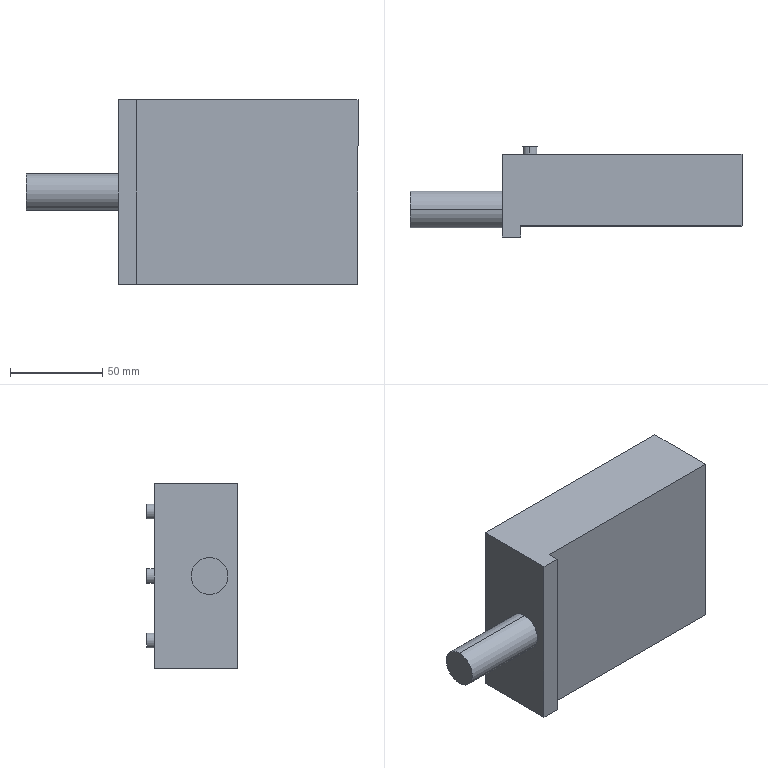Part | SolidWorks | features ICE 6, Extrusion 1, MirrorSolid 1 | 1 solid | 41 faces | box 180 x 49 x 100 mm | volume 529109 mm3 | plane 33 | cylinder 8 | commonest cylinder face diameters 8 x6 20 x2
STEP:
#1=CARTESIAN_POINT('',(-155.,0.,10.));
#2=VERTEX_POINT('',#1);
#3=CARTESIAN_POINT('',(-155.,0.,-10.));
#4=VERTEX_POINT('',#3);
#5=CARTESIAN_POINT('',(-155.,0.,0.));
#6=DIRECTION('',(1.,0.,0.));
#7=DIRECTION('',(0.,0.,-1.));
#8=AXIS2_PLACEMENT_3D('',#5,#6,#7);
#9=CIRCLE('',#8,10.);
#10=EDGE_CURVE('',#2,#4,#9,.T.);
#11=ORIENTED_EDGE('',*,*,#10,.T.);
#12=CARTESIAN_POINT('',(-105.,0.,-10.));
#13=VERTEX_POINT('',#12);
#14=CARTESIAN_POINT('',(-155.,0.,-10.));
#15=DIRECTION('',(1.,0.,0.));
#16=VECTOR('',#15,1000.);
#17=LINE('',#14,#16);
#18=EDGE_CURVE('',#4,#13,#17,.T.);
#19=ORIENTED_EDGE('',*,*,#18,.T.);
#20=CARTESIAN_POINT('',(-105.,0.,10.));
#21=VERTEX_POINT('',#20);
#22=CARTESIAN_POINT('',(-105.,0.,0.));
#23=DIRECTION('',(1.,0.,0.));
#24=DIRECTION('',(0.,0.,-1.));
#25=AXIS2_PLACEMENT_3D('',#22,#23,#24);
#26=CIRCLE('',#25,10.);
#27=EDGE_CURVE('',#21,#13,#26,.T.);
#28=ORIENTED_EDGE('',*,*,#27,.F.);
#29=CARTESIAN_POINT('',(-155.,0.,10.));
#30=DIRECTION('',(1.,0.,0.));
#31=VECTOR('',#30,1000.);
#32=LINE('',#29,#31);
#33=EDGE_CURVE('',#2,#21,#32,.T.);
#34=ORIENTED_EDGE('',*,*,#33,.F.);
#35=EDGE_LOOP('',(#11,#19,#28,#34));
#36=FACE_OUTER_BOUND('',#35,.T.);
#37=CARTESIAN_POINT('',(-155.,0.,0.));
#38=DIRECTION('',(1.,0.,0.));
#39=DIRECTION('',(0.,0.,1.));
#40=AXIS2_PLACEMENT_3D('',#37,#38,#39);
#41=CYLINDRICAL_SURFACE('',#40,10.);
#42=ADVANCED_FACE('',(#36),#41,.T.);
#43=CARTESIAN_POINT('',(-90.,34.,31.));
#44=VERTEX_POINT('',#43);
#45=CARTESIAN_POINT('',(-90.,34.,39.));
#46=VERTEX_POINT('',#45);
#47=CARTESIAN_POINT('',(-90.,34.,35.));
#48=DIRECTION('',(0.,-1.,0.));
#49=DIRECTION('',(0.,0.,1.));
#50=AXIS2_PLACEMENT_3D('',#47,#48,#49);
#51=CIRCLE('',#50,4.);
#52=EDGE_CURVE('',#44,#46,#51,.T.);
#53=ORIENTED_EDGE('',*,*,#52,.T.);
#54=CARTESIAN_POINT('',(-90.,30.,39.));
#55=VERTEX_POINT('',#54);
#56=CARTESIAN_POINT('',(-90.,34.,39.));
#57=DIRECTION('',(0.,-1.,0.));
#58=VECTOR('',#57,1000.);
#59=LINE('',#56,#58);
#60=EDGE_CURVE('',#46,#55,#59,.T.);
#61=ORIENTED_EDGE('',*,*,#60,.T.);
#62=CARTESIAN_POINT('',(-90.,30.,31.));
#63=VERTEX_POINT('',#62);
#64=CARTESIAN_POINT('',(-90.,30.,35.));
#65=DIRECTION('',(0.,-1.,0.));
#66=DIRECTION('',(0.,0.,1.));
#67=AXIS2_PLACEMENT_3D('',#64,#65,#66);
#68=CIRCLE('',#67,4.);
#69=EDGE_CURVE('',#63,#55,#68,.T.);
#70=ORIENTED_EDGE('',*,*,#69,.F.);
#71=CARTESIAN_POINT('',(-90.,34.,31.));
#72=DIRECTION('',(0.,-1.,0.));
#73=VECTOR('',#72,1000.);
#74=LINE('',#71,#73);
#75=EDGE_CURVE('',#44,#63,#74,.T.);
#76=ORIENTED_EDGE('',*,*,#75,.F.);
#77=EDGE_LOOP('',(#53,#61,#70,#76));
#78=FACE_OUTER_BOUND('',#77,.T.);
#79=CARTESIAN_POINT('',(-90.,34.,35.));
#80=DIRECTION('',(0.,-1.,0.));
#81=DIRECTION('',(0.,0.,-1.));
#82=AXIS2_PLACEMENT_3D('',#79,#80,#81);
#83=CYLINDRICAL_SURFACE('',#82,4.);
#84=ADVANCED_FACE('',(#78),#83,.T.);
#85=CARTESIAN_POINT('',(-90.,34.,-4.));
#86=VERTEX_POINT('',#85);
#87=CARTESIAN_POINT('',(-90.,34.,4.));
#88=VERTEX_POINT('',#87);
#89=CARTESIAN_POINT('',(-90.,34.,0.));
#90=DIRECTION('',(0.,-1.,0.));
#91=DIRECTION('',(0.,0.,1.));
#92=AXIS2_PLACEMENT_3D('',#89,#90,#91);
#93=CIRCLE('',#92,4.);
#94=EDGE_CURVE('',#86,#88,#93,.T.);
#95=ORIENTED_EDGE('',*,*,#94,.T.);
#96=CARTESIAN_POINT('',(-90.,30.,4.));
#97=VERTEX_POINT('',#96);
#98=CARTESIAN_POINT('',(-90.,34.,4.));
#99=DIRECTION('',(0.,-1.,0.));
#100=VECTOR('',#99,1000.);
#101=LINE('',#98,#100);
#102=EDGE_CURVE('',#88,#97,#101,.T.);
#103=ORIENTED_EDGE('',*,*,#102,.T.);
#104=CARTESIAN_POINT('',(-90.,30.,-4.));
#105=VERTEX_POINT('',#104);
#106=CARTESIAN_POINT('',(-90.,30.,0.));
#107=DIRECTION('',(0.,-1.,0.));
#108=DIRECTION('',(0.,0.,1.));
#109=AXIS2_PLACEMENT_3D('',#106,#107,#108);
#110=CIRCLE('',#109,4.);
#111=EDGE_CURVE('',#105,#97,#110,.T.);
#112=ORIENTED_EDGE('',*,*,#111,.F.);
#113=CARTESIAN_POINT('',(-90.,34.,-4.));
#114=DIRECTION('',(0.,-1.,0.));
#115=VECTOR('',#114,1000.);
#116=LINE('',#113,#115);
#117=EDGE_CURVE('',#86,#105,#116,.T.);
#118=ORIENTED_EDGE('',*,*,#117,.F.);
#119=EDGE_LOOP('',(#95,#103,#112,#118));
#120=FACE_OUTER_BOUND('',#119,.T.);
#121=CARTESIAN_POINT('',(-90.,34.,0.));
#122=DIRECTION('',(0.,-1.,0.));
#123=DIRECTION('',(0.,0.,-1.));
#124=AXIS2_PLACEMENT_3D('',#121,#122,#123);
#125=CYLINDRICAL_SURFACE('',#124,4.);
#126=ADVANCED_FACE('',(#120),#125,.T.);
#127=CARTESIAN_POINT('',(-90.,34.,-39.));
#128=VERTEX_POINT('',#127);
#129=CARTESIAN_POINT('',(-90.,34.,-31.));
#130=VERTEX_POINT('',#129);
#131=CARTESIAN_POINT('',(-90.,34.,-35.));
#132=DIRECTION('',(0.,-1.,0.));
#133=DIRECTION('',(0.,0.,1.));
#134=AXIS2_PLACEMENT_3D('',#131,#132,#133);
#135=CIRCLE('',#134,4.);
#136=EDGE_CURVE('',#128,#130,#135,.T.);
#137=ORIENTED_EDGE('',*,*,#136,.T.);
#138=CARTESIAN_POINT('',(-90.,30.,-31.));
#139=VERTEX_POINT('',#138);
#140=CARTESIAN_POINT('',(-90.,34.,-31.));
#141=DIRECTION('',(0.,-1.,0.));
#142=VECTOR('',#141,1000.);
#143=LINE('',#140,#142);
#144=EDGE_CURVE('',#130,#139,#143,.T.);
#145=ORIENTED_EDGE('',*,*,#144,.T.);
#146=CARTESIAN_POINT('',(-90.,30.,-39.));
#147=VERTEX_POINT('',#146);
#148=CARTESIAN_POINT('',(-90.,30.,-35.));
#149=DIRECTION('',(0.,-1.,0.));
#150=DIRECTION('',(0.,0.,1.));
#151=AXIS2_PLACEMENT_3D('',#148,#149,#150);
#152=CIRCLE('',#151,4.);
#153=EDGE_CURVE('',#147,#139,#152,.T.);
#154=ORIENTED_EDGE('',*,*,#153,.F.);
#155=CARTESIAN_POINT('',(-90.,34.,-39.));
#156=DIRECTION('',(0.,-1.,0.));
#157=VECTOR('',#156,1000.);
#158=LINE('',#155,#157);
#159=EDGE_CURVE('',#128,#147,#158,.T.);
#160=ORIENTED_EDGE('',*,*,#159,.F.);
#161=EDGE_LOOP('',(#137,#145,#154,#160));
#162=FACE_OUTER_BOUND('',#161,.T.);
#163=CARTESIAN_POINT('',(-90.,34.,-35.));
#164=DIRECTION('',(0.,-1.,0.));
#165=DIRECTION('',(0.,0.,-1.));
#166=AXIS2_PLACEMENT_3D('',#163,#164,#165);
#167=CYLINDRICAL_SURFACE('',#166,4.);
#168=ADVANCED_FACE('',(#162),#167,.T.);
#169=CARTESIAN_POINT('',(-105.,30.,50.));
#170=VERTEX_POINT('',#169);
#171=CARTESIAN_POINT('',(25.,30.,50.));
#172=VERTEX_POINT('',#171);
#173=CARTESIAN_POINT('',(-35.,30.,50.));
#174=DIRECTION('',(1.,0.,0.));
#175=VECTOR('',#174,1000.);
#176=LINE('',#173,#175);
#177=EDGE_CURVE('',#170,#172,#176,.T.);
#178=ORIENTED_EDGE('',*,*,#177,.T.);
#179=CARTESIAN_POINT('',(25.,30.,-50.));
#180=VERTEX_POINT('',#179);
#181=CARTESIAN_POINT('',(25.,30.,50.));
#182=DIRECTION('',(0.,0.,1.));
#183=VECTOR('',#182,1000.);
#184=LINE('',#181,#183);
#185=EDGE_CURVE('',#180,#172,#184,.T.);
#186=ORIENTED_EDGE('',*,*,#185,.F.);
#187=CARTESIAN_POINT('',(-105.,30.,-50.));
#188=VERTEX_POINT('',#187);
#189=CARTESIAN_POINT('',(-35.,30.,-50.));
#190=DIRECTION('',(-1.,0.,0.));
#191=VECTOR('',#190,1000.);
#192=LINE('',#189,#191);
#193=EDGE_CURVE('',#180,#188,#192,.T.);
#194=ORIENTED_EDGE('',*,*,#193,.T.);
#195=CARTESIAN_POINT('',(-105.,30.,-50.));
#196=DIRECTION('',(0.,0.,-1.));
#197=VECTOR('',#196,1000.);
#198=LINE('',#195,#197);
#199=EDGE_CURVE('',#170,#188,#198,.T.);
#200=ORIENTED_EDGE('',*,*,#199,.F.);
#201=EDGE_LOOP('',(#178,#186,#194,#200));
#202=FACE_OUTER_BOUND('',#201,.T.);
#203=ORIENTED_EDGE('',*,*,#111,.T.);
#204=CARTESIAN_POINT('',(-90.,30.,0.));
#205=DIRECTION('',(0.,-1.,0.));
#206=DIRECTION('',(0.,0.,1.));
#207=AXIS2_PLACEMENT_3D('',#204,#205,#206);
#208=CIRCLE('',#207,4.);
#209=EDGE_CURVE('',#97,#105,#208,.T.);
#210=ORIENTED_EDGE('',*,*,#209,.T.);
#211=EDGE_LOOP('',(#203,#210));
#212=FACE_BOUND('',#211,.T.);
#213=ORIENTED_EDGE('',*,*,#153,.T.);
#214=CARTESIAN_POINT('',(-90.,30.,-35.));
#215=DIRECTION('',(0.,-1.,0.));
#216=DIRECTION('',(0.,0.,1.));
#217=AXIS2_PLACEMENT_3D('',#214,#215,#216);
#218=CIRCLE('',#217,4.);
#219=EDGE_CURVE('',#139,#147,#218,.T.);
#220=ORIENTED_EDGE('',*,*,#219,.T.);
#221=EDGE_LOOP('',(#213,#220));
#222=FACE_BOUND('',#221,.T.);
#223=ORIENTED_EDGE('',*,*,#69,.T.);
#224=CARTESIAN_POINT('',(-90.,30.,35.));
#225=DIRECTION('',(0.,-1.,0.));
#226=DIRECTION('',(0.,0.,1.));
#227=AXIS2_PLACEMENT_3D('',#224,#225,#226);
#228=CIRCLE('',#227,4.);
#229=EDGE_CURVE('',#55,#63,#228,.T.);
#230=ORIENTED_EDGE('',*,*,#229,.T.);
#231=EDGE_LOOP('',(#223,#230));
#232=FACE_BOUND('',#231,.T.);
#233=CARTESIAN_POINT('',(0.,30.,0.));
#234=DIRECTION('',(0.,1.,0.));
#235=DIRECTION('',(0.,0.,1.));
#236=AXIS2_PLACEMENT_3D('',#233,#234,#235);
#237=PLANE('',#236);
#238=ADVANCED_FACE('',(#202,#212,#222,#232),#237,.T.);
#239=CARTESIAN_POINT('',(-95.,-9.,-50.));
#240=VERTEX_POINT('',#239);
#241=CARTESIAN_POINT('',(25.,-9.,-50.));
#242=VERTEX_POINT('',#241);
#243=CARTESIAN_POINT('',(-35.,-9.,-50.));
#244=DIRECTION('',(1.,0.,0.));
#245=VECTOR('',#244,1000.);
#246=LINE('',#243,#245);
#247=EDGE_CURVE('',#240,#242,#246,.T.);
#248=ORIENTED_EDGE('',*,*,#247,.F.);
#249=CARTESIAN_POINT('',(-95.,-15.,-50.));
#250=VERTEX_POINT('',#249);
#251=CARTESIAN_POINT('',(-95.,-15.,-50.));
#252=DIRECTION('',(0.,1.,0.));
#253=VECTOR('',#252,1000.);
#254=LINE('',#251,#253);
#255=EDGE_CURVE('',#250,#240,#254,.T.);
#256=ORIENTED_EDGE('',*,*,#255,.F.);
#257=CARTESIAN_POINT('',(-105.,-15.,-50.));
#258=VERTEX_POINT('',#257);
#259=CARTESIAN_POINT('',(-35.,-15.,-50.));
#260=DIRECTION('',(1.,0.,0.));
#261=VECTOR('',#260,1000.);
#262=LINE('',#259,#261);
#263=EDGE_CURVE('',#258,#250,#262,.T.);
#264=ORIENTED_EDGE('',*,*,#263,.F.);
#265=CARTESIAN_POINT('',(-105.,30.,-50.));
#266=DIRECTION('',(0.,-1.,0.));
#267=VECTOR('',#266,1000.);
#268=LINE('',#265,#267);
#269=EDGE_CURVE('',#188,#258,#268,.T.);
#270=ORIENTED_EDGE('',*,*,#269,.F.);
#271=ORIENTED_EDGE('',*,*,#193,.F.);
#272=CARTESIAN_POINT('',(25.,30.,-50.));
#273=DIRECTION('',(0.,1.,0.));
#274=VECTOR('',#273,1000.);
#275=LINE('',#272,#274);
#276=EDGE_CURVE('',#242,#180,#275,.T.);
#277=ORIENTED_EDGE('',*,*,#276,.F.);
#278=EDGE_LOOP('',(#248,#256,#264,#270,#271,#277));
#279=FACE_OUTER_BOUND('',#278,.T.);
#280=CARTESIAN_POINT('',(-35.,30.,-50.));
#281=DIRECTION('',(0.,0.,1.));
#282=DIRECTION('',(1.,0.,0.));
#283=AXIS2_PLACEMENT_3D('',#280,#281,#282);
#284=PLANE('',#283);
#285=ADVANCED_FACE('',(#279),#284,.F.);
#286=CARTESIAN_POINT('',(-95.,-15.,50.));
#287=VERTEX_POINT('',#286);
#288=CARTESIAN_POINT('',(-105.,-15.,50.));
#289=VERTEX_POINT('',#288);
#290=CARTESIAN_POINT('',(-35.,-15.,50.));
#291=DIRECTION('',(-1.,0.,0.));
#292=VECTOR('',#291,1000.);
#293=LINE('',#290,#292);
#294=EDGE_CURVE('',#287,#289,#293,.T.);
#295=ORIENTED_EDGE('',*,*,#294,.F.);
#296=CARTESIAN_POINT('',(-95.,-9.,50.));
#297=VERTEX_POINT('',#296);
#298=CARTESIAN_POINT('',(-95.,-15.,50.));
#299=DIRECTION('',(0.,-1.,0.));
#300=VECTOR('',#299,1000.);
#301=LINE('',#298,#300);
#302=EDGE_CURVE('',#297,#287,#301,.T.);
#303=ORIENTED_EDGE('',*,*,#302,.F.);
#304=CARTESIAN_POINT('',(25.,-9.,50.));
#305=VERTEX_POINT('',#304);
#306=CARTESIAN_POINT('',(-35.,-9.,50.));
#307=DIRECTION('',(-1.,0.,0.));
#308=VECTOR('',#307,1000.);
#309=LINE('',#306,#308);
#310=EDGE_CURVE('',#305,#297,#309,.T.);
#311=ORIENTED_EDGE('',*,*,#310,.F.);
#312=CARTESIAN_POINT('',(25.,30.,50.));
#313=DIRECTION('',(0.,-1.,0.));
#314=VECTOR('',#313,1000.);
#315=LINE('',#312,#314);
#316=EDGE_CURVE('',#172,#305,#315,.T.);
#317=ORIENTED_EDGE('',*,*,#316,.F.);
#318=ORIENTED_EDGE('',*,*,#177,.F.);
#319=CARTESIAN_POINT('',(-105.,30.,50.));
#320=DIRECTION('',(0.,-1.,0.));
#321=VECTOR('',#320,1000.);
#322=LINE('',#319,#321);
#323=EDGE_CURVE('',#170,#289,#322,.T.);
#324=ORIENTED_EDGE('',*,*,#323,.T.);
#325=EDGE_LOOP('',(#295,#303,#311,#317,#318,#324));
#326=FACE_OUTER_BOUND('',#325,.T.);
#327=CARTESIAN_POINT('',(-35.,30.,50.));
#328=DIRECTION('',(0.,0.,-1.));
#329=DIRECTION('',(-1.,0.,0.));
#330=AXIS2_PLACEMENT_3D('',#327,#328,#329);
#331=PLANE('',#330);
#332=ADVANCED_FACE('',(#326),#331,.F.);
#333=CARTESIAN_POINT('',(-95.,-15.,-50.001));
#334=DIRECTION('',(0.,0.,1.));
#335=VECTOR('',#334,1000.);
#336=LINE('',#333,#335);
#337=EDGE_CURVE('',#250,#287,#336,.T.);
#338=ORIENTED_EDGE('',*,*,#337,.T.);
#339=ORIENTED_EDGE('',*,*,#294,.T.);
#340=CARTESIAN_POINT('',(-105.,-15.,50.));
#341=DIRECTION('',(0.,0.,1.));
#342=VECTOR('',#341,1000.);
#343=LINE('',#340,#342);
#344=EDGE_CURVE('',#258,#289,#343,.T.);
#345=ORIENTED_EDGE('',*,*,#344,.F.);
#346=ORIENTED_EDGE('',*,*,#263,.T.);
#347=EDGE_LOOP('',(#338,#339,#345,#346));
#348=FACE_OUTER_BOUND('',#347,.T.);
#349=CARTESIAN_POINT('',(0.,-15.,0.));
#350=DIRECTION('',(0.,-1.,0.));
#351=DIRECTION('',(0.,0.,-1.));
#352=AXIS2_PLACEMENT_3D('',#349,#350,#351);
#353=PLANE('',#352);
#354=ADVANCED_FACE('',(#348),#353,.T.);
#355=ORIENTED_EDGE('',*,*,#344,.T.);
#356=ORIENTED_EDGE('',*,*,#323,.F.);
#357=ORIENTED_EDGE('',*,*,#199,.T.);
#358=ORIENTED_EDGE('',*,*,#269,.T.);
#359=EDGE_LOOP('',(#355,#356,#357,#358));
#360=FACE_OUTER_BOUND('',#359,.T.);
#361=ORIENTED_EDGE('',*,*,#27,.T.);
#362=CARTESIAN_POINT('',(-105.,0.,0.));
#363=DIRECTION('',(1.,0.,0.));
#364=DIRECTION('',(0.,0.,-1.));
#365=AXIS2_PLACEMENT_3D('',#362,#363,#364);
#366=CIRCLE('',#365,10.);
#367=EDGE_CURVE('',#13,#21,#366,.T.);
#368=ORIENTED_EDGE('',*,*,#367,.T.);
#369=EDGE_LOOP('',(#361,#368));
#370=FACE_BOUND('',#369,.T.);
#371=CARTESIAN_POINT('',(-105.,30.,-50.));
#372=DIRECTION('',(1.,0.,0.));
#373=DIRECTION('',(0.,0.,1.));
#374=AXIS2_PLACEMENT_3D('',#371,#372,#373);
#375=PLANE('',#374);
#376=ADVANCED_FACE('',(#360,#370),#375,.F.);
#377=ORIENTED_EDGE('',*,*,#136,.F.);
#378=CARTESIAN_POINT('',(-90.,34.,-35.));
#379=DIRECTION('',(0.,-1.,0.));
#380=DIRECTION('',(0.,0.,1.));
#381=AXIS2_PLACEMENT_3D('',#378,#379,#380);
#382=CIRCLE('',#381,4.);
#383=EDGE_CURVE('',#130,#128,#382,.T.);
#384=ORIENTED_EDGE('',*,*,#383,.F.);
#385=EDGE_LOOP('',(#377,#384));
#386=FACE_OUTER_BOUND('',#385,.T.);
#387=CARTESIAN_POINT('',(-91.913,34.,-33.535));
#388=VERTEX_POINT('',#387);
#389=CARTESIAN_POINT('',(-92.226,34.,-35.924));
#390=VERTEX_POINT('',#389);
#391=CARTESIAN_POINT('',(-91.913,34.,-33.535));
#392=DIRECTION('',(-0.1297,0.,-0.9916));
#393=VECTOR('',#392,1000.);
#394=LINE('',#391,#393);
#395=EDGE_CURVE('',#388,#390,#394,.T.);
#396=ORIENTED_EDGE('',*,*,#395,.T.);
#397=CARTESIAN_POINT('',(-90.312,34.,-37.389));
#398=VERTEX_POINT('',#397);
#399=CARTESIAN_POINT('',(-92.226,34.,-35.924));
#400=DIRECTION('',(0.7939,0.,-0.6081));
#401=VECTOR('',#400,1000.);
#402=LINE('',#399,#401);
#403=EDGE_CURVE('',#390,#398,#402,.T.);
#404=ORIENTED_EDGE('',*,*,#403,.T.);
#405=CARTESIAN_POINT('',(-88.087,34.,-36.465));
#406=VERTEX_POINT('',#405);
#407=CARTESIAN_POINT('',(-90.312,34.,-37.389));
#408=DIRECTION('',(0.9235,0.,0.3835));
#409=VECTOR('',#408,1000.);
#410=LINE('',#407,#409);
#411=EDGE_CURVE('',#398,#406,#410,.T.);
#412=ORIENTED_EDGE('',*,*,#411,.T.);
#413=CARTESIAN_POINT('',(-87.774,34.,-34.076));
#414=VERTEX_POINT('',#413);
#415=CARTESIAN_POINT('',(-88.087,34.,-36.465));
#416=DIRECTION('',(0.1297,0.,0.9916));
#417=VECTOR('',#416,1000.);
#418=LINE('',#415,#417);
#419=EDGE_CURVE('',#406,#414,#418,.T.);
#420=ORIENTED_EDGE('',*,*,#419,.T.);
#421=CARTESIAN_POINT('',(-89.688,34.,-32.611));
#422=VERTEX_POINT('',#421);
#423=CARTESIAN_POINT('',(-87.774,34.,-34.076));
#424=DIRECTION('',(-0.7939,0.,0.6081));
#425=VECTOR('',#424,1000.);
#426=LINE('',#423,#425);
#427=EDGE_CURVE('',#414,#422,#426,.T.);
#428=ORIENTED_EDGE('',*,*,#427,.T.);
#429=CARTESIAN_POINT('',(-89.688,34.,-32.611));
#430=DIRECTION('',(-0.9235,0.,-0.3835));
#431=VECTOR('',#430,1000.);
#432=LINE('',#429,#431);
#433=EDGE_CURVE('',#422,#388,#432,.T.);
#434=ORIENTED_EDGE('',*,*,#433,.T.);
#435=EDGE_LOOP('',(#396,#404,#412,#420,#428,#434));
#436=FACE_BOUND('',#435,.T.);
#437=CARTESIAN_POINT('',(-90.,34.,-35.));
#438=DIRECTION('',(0.,1.,0.));
#439=DIRECTION('',(0.,0.,1.));
#440=AXIS2_PLACEMENT_3D('',#437,#438,#439);
#441=PLANE('',#440);
#442=ADVANCED_FACE('',(#386,#436),#441,.T.);
#443=ORIENTED_EDGE('',*,*,#144,.F.);
#444=ORIENTED_EDGE('',*,*,#383,.T.);
#445=ORIENTED_EDGE('',*,*,#159,.T.);
#446=ORIENTED_EDGE('',*,*,#219,.F.);
#447=EDGE_LOOP('',(#443,#444,#445,#446));
#448=FACE_OUTER_BOUND('',#447,.T.);
#449=CARTESIAN_POINT('',(-90.,34.,-35.));
#450=DIRECTION('',(0.,-1.,0.));
#451=DIRECTION('',(0.,0.,-1.));
#452=AXIS2_PLACEMENT_3D('',#449,#450,#451);
#453=CYLINDRICAL_SURFACE('',#452,4.);
#454=ADVANCED_FACE('',(#448),#453,.T.);
#455=CARTESIAN_POINT('',(-89.688,30.,-32.611));
#456=VERTEX_POINT('',#455);
#457=CARTESIAN_POINT('',(-91.913,30.,-33.535));
#458=VERTEX_POINT('',#457);
#459=CARTESIAN_POINT('',(-89.688,30.,-32.611));
#460=DIRECTION('',(-0.9235,0.,-0.3835));
#461=VECTOR('',#460,1000.);
#462=LINE('',#459,#461);
#463=EDGE_CURVE('',#456,#458,#462,.T.);
#464=ORIENTED_EDGE('',*,*,#463,.T.);
#465=CARTESIAN_POINT('',(-91.913,34.,-33.535));
#466=DIRECTION('',(0.,-1.,0.));
#467=VECTOR('',#466,1000.);
#468=LINE('',#465,#467);
#469=EDGE_CURVE('',#388,#458,#468,.T.);
#470=ORIENTED_EDGE('',*,*,#469,.F.);
#471=ORIENTED_EDGE('',*,*,#433,.F.);
#472=CARTESIAN_POINT('',(-89.688,34.,-32.611));
#473=DIRECTION('',(0.,-1.,0.));
#474=VECTOR('',#473,1000.);
#475=LINE('',#472,#474);
#476=EDGE_CURVE('',#422,#456,#475,.T.);
#477=ORIENTED_EDGE('',*,*,#476,.T.);
#478=EDGE_LOOP('',(#464,#470,#471,#477));
#479=FACE_OUTER_BOUND('',#478,.T.);
#480=CARTESIAN_POINT('',(-89.688,34.,-32.611));
#481=DIRECTION('',(0.3835,0.,-0.9235));
#482=DIRECTION('',(0.9235,0.,0.3835));
#483=AXIS2_PLACEMENT_3D('',#480,#481,#482);
#484=PLANE('',#483);
#485=ADVANCED_FACE('',(#479),#484,.T.);
#486=CARTESIAN_POINT('',(-92.226,30.,-35.924));
#487=VERTEX_POINT('',#486);
#488=CARTESIAN_POINT('',(-91.913,30.,-33.535));
#489=DIRECTION('',(-0.1297,0.,-0.9916));
#490=VECTOR('',#489,1000.);
#491=LINE('',#488,#490);
#492=EDGE_CURVE('',#458,#487,#491,.T.);
#493=ORIENTED_EDGE('',*,*,#492,.T.);
#494=CARTESIAN_POINT('',(-92.226,34.,-35.924));
#495=DIRECTION('',(0.,-1.,0.));
#496=VECTOR('',#495,1000.);
#497=LINE('',#494,#496);
#498=EDGE_CURVE('',#390,#487,#497,.T.);
#499=ORIENTED_EDGE('',*,*,#498,.F.);
#500=ORIENTED_EDGE('',*,*,#395,.F.);
#501=ORIENTED_EDGE('',*,*,#469,.T.);
#502=EDGE_LOOP('',(#493,#499,#500,#501));
#503=FACE_OUTER_BOUND('',#502,.T.);
#504=CARTESIAN_POINT('',(-91.913,34.,-33.535));
#505=DIRECTION('',(0.9916,0.,-0.1297));
#506=DIRECTION('',(0.1297,0.,0.9916));
#507=AXIS2_PLACEMENT_3D('',#504,#505,#506);
#508=PLANE('',#507);
#509=ADVANCED_FACE('',(#503),#508,.T.);
#510=CARTESIAN_POINT('',(-90.312,30.,-37.389));
#511=VERTEX_POINT('',#510);
#512=CARTESIAN_POINT('',(-92.226,30.,-35.924));
#513=DIRECTION('',(0.7939,0.,-0.6081));
#514=VECTOR('',#513,1000.);
#515=LINE('',#512,#514);
#516=EDGE_CURVE('',#487,#511,#515,.T.);
#517=ORIENTED_EDGE('',*,*,#516,.T.);
#518=CARTESIAN_POINT('',(-90.312,34.,-37.389));
#519=DIRECTION('',(0.,-1.,0.));
#520=VECTOR('',#519,1000.);
#521=LINE('',#518,#520);
#522=EDGE_CURVE('',#398,#511,#521,.T.);
#523=ORIENTED_EDGE('',*,*,#522,.F.);
#524=ORIENTED_EDGE('',*,*,#403,.F.);
#525=ORIENTED_EDGE('',*,*,#498,.T.);
#526=EDGE_LOOP('',(#517,#523,#524,#525));
#527=FACE_OUTER_BOUND('',#526,.T.);
#528=CARTESIAN_POINT('',(-92.226,34.,-35.924));
#529=DIRECTION('',(0.6081,0.,0.7939));
#530=DIRECTION('',(-0.7939,0.,0.6081));
#531=AXIS2_PLACEMENT_3D('',#528,#529,#530);
#532=PLANE('',#531);
#533=ADVANCED_FACE('',(#527),#532,.T.);
#534=CARTESIAN_POINT('',(-88.087,30.,-36.465));
#535=VERTEX_POINT('',#534);
#536=CARTESIAN_POINT('',(-90.312,30.,-37.389));
#537=DIRECTION('',(0.9235,0.,0.3835));
#538=VECTOR('',#537,1000.);
#539=LINE('',#536,#538);
#540=EDGE_CURVE('',#511,#535,#539,.T.);
#541=ORIENTED_EDGE('',*,*,#540,.T.);
#542=CARTESIAN_POINT('',(-88.087,34.,-36.465));
#543=DIRECTION('',(0.,-1.,0.));
#544=VECTOR('',#543,1000.);
#545=LINE('',#542,#544);
#546=EDGE_CURVE('',#406,#535,#545,.T.);
#547=ORIENTED_EDGE('',*,*,#546,.F.);
#548=ORIENTED_EDGE('',*,*,#411,.F.);
#549=ORIENTED_EDGE('',*,*,#522,.T.);
#550=EDGE_LOOP('',(#541,#547,#548,#549));
#551=FACE_OUTER_BOUND('',#550,.T.);
#552=CARTESIAN_POINT('',(-90.312,34.,-37.389));
#553=DIRECTION('',(-0.3835,0.,0.9235));
#554=DIRECTION('',(-0.9235,0.,-0.3835));
#555=AXIS2_PLACEMENT_3D('',#552,#553,#554);
#556=PLANE('',#555);
#557=ADVANCED_FACE('',(#551),#556,.T.);
#558=CARTESIAN_POINT('',(-87.774,30.,-34.076));
#559=VERTEX_POINT('',#558);
#560=CARTESIAN_POINT('',(-88.087,30.,-36.465));
#561=DIRECTION('',(0.1297,0.,0.9916));
#562=VECTOR('',#561,1000.);
#563=LINE('',#560,#562);
#564=EDGE_CURVE('',#535,#559,#563,.T.);
#565=ORIENTED_EDGE('',*,*,#564,.T.);
#566=CARTESIAN_POINT('',(-87.774,34.,-34.076));
#567=DIRECTION('',(0.,-1.,0.));
#568=VECTOR('',#567,1000.);
#569=LINE('',#566,#568);
#570=EDGE_CURVE('',#414,#559,#569,.T.);
#571=ORIENTED_EDGE('',*,*,#570,.F.);
#572=ORIENTED_EDGE('',*,*,#419,.F.);
#573=ORIENTED_EDGE('',*,*,#546,.T.);
#574=EDGE_LOOP('',(#565,#571,#572,#573));
#575=FACE_OUTER_BOUND('',#574,.T.);
#576=CARTESIAN_POINT('',(-88.087,34.,-36.465));
#577=DIRECTION('',(-0.9916,0.,0.1297));
#578=DIRECTION('',(-0.1297,0.,-0.9916));
#579=AXIS2_PLACEMENT_3D('',#576,#577,#578);
#580=PLANE('',#579);
#581=ADVANCED_FACE('',(#575),#580,.T.);
#582=CARTESIAN_POINT('',(-87.774,30.,-34.076));
#583=DIRECTION('',(-0.7939,0.,0.6081));
#584=VECTOR('',#583,1000.);
#585=LINE('',#582,#584);
#586=EDGE_CURVE('',#559,#456,#585,.T.);
#587=ORIENTED_EDGE('',*,*,#586,.T.);
#588=ORIENTED_EDGE('',*,*,#476,.F.);
#589=ORIENTED_EDGE('',*,*,#427,.F.);
#590=ORIENTED_EDGE('',*,*,#570,.T.);
#591=EDGE_LOOP('',(#587,#588,#589,#590));
#592=FACE_OUTER_BOUND('',#591,.T.);
#593=CARTESIAN_POINT('',(-87.774,34.,-34.076));
#594=DIRECTION('',(-0.6081,0.,-0.7939));
#595=DIRECTION('',(0.7939,0.,-0.6081));
#596=AXIS2_PLACEMENT_3D('',#593,#594,#595);
#597=PLANE('',#596);
#598=ADVANCED_FACE('',(#592),#597,.T.);
#599=ORIENTED_EDGE('',*,*,#463,.F.);
#600=ORIENTED_EDGE('',*,*,#586,.F.);
#601=ORIENTED_EDGE('',*,*,#564,.F.);
#602=ORIENTED_EDGE('',*,*,#540,.F.);
#603=ORIENTED_EDGE('',*,*,#516,.F.);
#604=ORIENTED_EDGE('',*,*,#492,.F.);
#605=EDGE_LOOP('',(#599,#600,#601,#602,#603,#604));
#606=FACE_OUTER_BOUND('',#605,.T.);
#607=CARTESIAN_POINT('',(-70.,30.,0.));
#608=DIRECTION('',(0.,1.,0.));
#609=DIRECTION('',(0.,0.,1.));
#610=AXIS2_PLACEMENT_3D('',#607,#608,#609);
#611=PLANE('',#610);
#612=ADVANCED_FACE('',(#606),#611,.T.);
#613=ORIENTED_EDGE('',*,*,#94,.F.);
#614=CARTESIAN_POINT('',(-90.,34.,0.));
#615=DIRECTION('',(0.,-1.,0.));
#616=DIRECTION('',(0.,0.,1.));
#617=AXIS2_PLACEMENT_3D('',#614,#615,#616);
#618=CIRCLE('',#617,4.);
#619=EDGE_CURVE('',#88,#86,#618,.T.);
#620=ORIENTED_EDGE('',*,*,#619,.F.);
#621=EDGE_LOOP('',(#613,#620));
#622=FACE_OUTER_BOUND('',#621,.T.);
#623=CARTESIAN_POINT('',(-91.913,34.,1.47));
#624=VERTEX_POINT('',#623);
#625=CARTESIAN_POINT('',(-92.23,34.,-0.9217));
#626=VERTEX_POINT('',#625);
#627=CARTESIAN_POINT('',(-91.913,34.,1.47));
#628=DIRECTION('',(-0.1313,0.,-0.9913));
#629=VECTOR('',#628,1000.);
#630=LINE('',#627,#629);
#631=EDGE_CURVE('',#624,#626,#630,.T.);
#632=ORIENTED_EDGE('',*,*,#631,.T.);
#633=CARTESIAN_POINT('',(-90.317,34.,-2.392));
#634=VERTEX_POINT('',#633);
#635=CARTESIAN_POINT('',(-92.23,34.,-0.9217));
#636=DIRECTION('',(0.7929,0.,-0.6094));
#637=VECTOR('',#636,1000.);
#638=LINE('',#635,#637);
#639=EDGE_CURVE('',#626,#634,#638,.T.);
#640=ORIENTED_EDGE('',*,*,#639,.T.);
#641=CARTESIAN_POINT('',(-88.087,34.,-1.47));
#642=VERTEX_POINT('',#641);
#643=CARTESIAN_POINT('',(-90.317,34.,-2.392));
#644=DIRECTION('',(0.9242,0.,0.382));
#645=VECTOR('',#644,1000.);
#646=LINE('',#643,#645);
#647=EDGE_CURVE('',#634,#642,#646,.T.);
#648=ORIENTED_EDGE('',*,*,#647,.T.);
#649=CARTESIAN_POINT('',(-87.77,34.,0.9217));
#650=VERTEX_POINT('',#649);
#651=CARTESIAN_POINT('',(-88.087,34.,-1.47));
#652=DIRECTION('',(0.1313,0.,0.9913));
#653=VECTOR('',#652,1000.);
#654=LINE('',#651,#653);
#655=EDGE_CURVE('',#642,#650,#654,.T.);
#656=ORIENTED_EDGE('',*,*,#655,.T.);
#657=CARTESIAN_POINT('',(-89.683,34.,2.392));
#658=VERTEX_POINT('',#657);
#659=CARTESIAN_POINT('',(-87.77,34.,0.9217));
#660=DIRECTION('',(-0.7929,0.,0.6094));
#661=VECTOR('',#660,1000.);
#662=LINE('',#659,#661);
#663=EDGE_CURVE('',#650,#658,#662,.T.);
#664=ORIENTED_EDGE('',*,*,#663,.T.);
#665=CARTESIAN_POINT('',(-89.683,34.,2.392));
#666=DIRECTION('',(-0.9242,0.,-0.382));
#667=VECTOR('',#666,1000.);
#668=LINE('',#665,#667);
#669=EDGE_CURVE('',#658,#624,#668,.T.);
#670=ORIENTED_EDGE('',*,*,#669,.T.);
#671=EDGE_LOOP('',(#632,#640,#648,#656,#664,#670));
#672=FACE_BOUND('',#671,.T.);
#673=CARTESIAN_POINT('',(-90.,34.,0.));
#674=DIRECTION('',(0.,1.,0.));
#675=DIRECTION('',(0.,0.,1.));
#676=AXIS2_PLACEMENT_3D('',#673,#674,#675);
#677=PLANE('',#676);
#678=ADVANCED_FACE('',(#622,#672),#677,.T.);
#679=ORIENTED_EDGE('',*,*,#102,.F.);
#680=ORIENTED_EDGE('',*,*,#619,.T.);
#681=ORIENTED_EDGE('',*,*,#117,.T.);
#682=ORIENTED_EDGE('',*,*,#209,.F.);
#683=EDGE_LOOP('',(#679,#680,#681,#682));
#684=FACE_OUTER_BOUND('',#683,.T.);
#685=CARTESIAN_POINT('',(-90.,34.,0.));
#686=DIRECTION('',(0.,-1.,0.));
#687=DIRECTION('',(0.,0.,-1.));
#688=AXIS2_PLACEMENT_3D('',#685,#686,#687);
#689=CYLINDRICAL_SURFACE('',#688,4.);
#690=ADVANCED_FACE('',(#684),#689,.T.);
#691=CARTESIAN_POINT('',(-89.683,30.,2.392));
#692=VERTEX_POINT('',#691);
#693=CARTESIAN_POINT('',(-91.913,30.,1.47));
#694=VERTEX_POINT('',#693);
#695=CARTESIAN_POINT('',(-89.683,30.,2.392));
#696=DIRECTION('',(-0.9242,0.,-0.382));
#697=VECTOR('',#696,1000.);
#698=LINE('',#695,#697);
#699=EDGE_CURVE('',#692,#694,#698,.T.);
#700=ORIENTED_EDGE('',*,*,#699,.T.);
#701=CARTESIAN_POINT('',(-91.913,34.,1.47));
#702=DIRECTION('',(0.,-1.,0.));
#703=VECTOR('',#702,1000.);
#704=LINE('',#701,#703);
#705=EDGE_CURVE('',#624,#694,#704,.T.);
#706=ORIENTED_EDGE('',*,*,#705,.F.);
#707=ORIENTED_EDGE('',*,*,#669,.F.);
#708=CARTESIAN_POINT('',(-89.683,34.,2.392));
#709=DIRECTION('',(0.,-1.,0.));
#710=VECTOR('',#709,1000.);
#711=LINE('',#708,#710);
#712=EDGE_CURVE('',#658,#692,#711,.T.);
#713=ORIENTED_EDGE('',*,*,#712,.T.);
#714=EDGE_LOOP('',(#700,#706,#707,#713));
#715=FACE_OUTER_BOUND('',#714,.T.);
#716=CARTESIAN_POINT('',(-89.683,34.,2.392));
#717=DIRECTION('',(0.382,0.,-0.9242));
#718=DIRECTION('',(0.9242,0.,0.382));
#719=AXIS2_PLACEMENT_3D('',#716,#717,#718);
#720=PLANE('',#719);
#721=ADVANCED_FACE('',(#715),#720,.T.);
#722=CARTESIAN_POINT('',(-92.23,30.,-0.9217));
#723=VERTEX_POINT('',#722);
#724=CARTESIAN_POINT('',(-91.913,30.,1.47));
#725=DIRECTION('',(-0.1313,0.,-0.9913));
#726=VECTOR('',#725,1000.);
#727=LINE('',#724,#726);
#728=EDGE_CURVE('',#694,#723,#727,.T.);
#729=ORIENTED_EDGE('',*,*,#728,.T.);
#730=CARTESIAN_POINT('',(-92.23,34.,-0.9217));
#731=DIRECTION('',(0.,-1.,0.));
#732=VECTOR('',#731,1000.);
#733=LINE('',#730,#732);
#734=EDGE_CURVE('',#626,#723,#733,.T.);
#735=ORIENTED_EDGE('',*,*,#734,.F.);
#736=ORIENTED_EDGE('',*,*,#631,.F.);
#737=ORIENTED_EDGE('',*,*,#705,.T.);
#738=EDGE_LOOP('',(#729,#735,#736,#737));
#739=FACE_OUTER_BOUND('',#738,.T.);
#740=CARTESIAN_POINT('',(-91.913,34.,1.47));
#741=DIRECTION('',(0.9913,0.,-0.1313));
#742=DIRECTION('',(0.1313,0.,0.9913));
#743=AXIS2_PLACEMENT_3D('',#740,#741,#742);
#744=PLANE('',#743);
#745=ADVANCED_FACE('',(#739),#744,.T.);
#746=CARTESIAN_POINT('',(-90.317,30.,-2.392));
#747=VERTEX_POINT('',#746);
#748=CARTESIAN_POINT('',(-92.23,30.,-0.9217));
#749=DIRECTION('',(0.7929,0.,-0.6094));
#750=VECTOR('',#749,1000.);
#751=LINE('',#748,#750);
#752=EDGE_CURVE('',#723,#747,#751,.T.);
#753=ORIENTED_EDGE('',*,*,#752,.T.);
#754=CARTESIAN_POINT('',(-90.317,34.,-2.392));
#755=DIRECTION('',(0.,-1.,0.));
#756=VECTOR('',#755,1000.);
#757=LINE('',#754,#756);
#758=EDGE_CURVE('',#634,#747,#757,.T.);
#759=ORIENTED_EDGE('',*,*,#758,.F.);
#760=ORIENTED_EDGE('',*,*,#639,.F.);
#761=ORIENTED_EDGE('',*,*,#734,.T.);
#762=EDGE_LOOP('',(#753,#759,#760,#761));
#763=FACE_OUTER_BOUND('',#762,.T.);
#764=CARTESIAN_POINT('',(-92.23,34.,-0.9217));
#765=DIRECTION('',(0.6094,0.,0.7929));
#766=DIRECTION('',(-0.7929,0.,0.6094));
#767=AXIS2_PLACEMENT_3D('',#764,#765,#766);
#768=PLANE('',#767);
#769=ADVANCED_FACE('',(#763),#768,.T.);
#770=CARTESIAN_POINT('',(-88.087,30.,-1.47));
#771=VERTEX_POINT('',#770);
#772=CARTESIAN_POINT('',(-90.317,30.,-2.392));
#773=DIRECTION('',(0.9242,0.,0.382));
#774=VECTOR('',#773,1000.);
#775=LINE('',#772,#774);
#776=EDGE_CURVE('',#747,#771,#775,.T.);
#777=ORIENTED_EDGE('',*,*,#776,.T.);
#778=CARTESIAN_POINT('',(-88.087,34.,-1.47));
#779=DIRECTION('',(0.,-1.,0.));
#780=VECTOR('',#779,1000.);
#781=LINE('',#778,#780);
#782=EDGE_CURVE('',#642,#771,#781,.T.);
#783=ORIENTED_EDGE('',*,*,#782,.F.);
#784=ORIENTED_EDGE('',*,*,#647,.F.);
#785=ORIENTED_EDGE('',*,*,#758,.T.);
#786=EDGE_LOOP('',(#777,#783,#784,#785));
#787=FACE_OUTER_BOUND('',#786,.T.);
#788=CARTESIAN_POINT('',(-90.317,34.,-2.392));
#789=DIRECTION('',(-0.382,0.,0.9242));
#790=DIRECTION('',(-0.9242,0.,-0.382));
#791=AXIS2_PLACEMENT_3D('',#788,#789,#790);
#792=PLANE('',#791);
#793=ADVANCED_FACE('',(#787),#792,.T.);
#794=CARTESIAN_POINT('',(-87.77,30.,0.9217));
#795=VERTEX_POINT('',#794);
#796=CARTESIAN_POINT('',(-88.087,30.,-1.47));
#797=DIRECTION('',(0.1313,0.,0.9913));
#798=VECTOR('',#797,1000.);
#799=LINE('',#796,#798);
#800=EDGE_CURVE('',#771,#795,#799,.T.);
#801=ORIENTED_EDGE('',*,*,#800,.T.);
#802=CARTESIAN_POINT('',(-87.77,34.,0.9217));
#803=DIRECTION('',(0.,-1.,0.));
#804=VECTOR('',#803,1000.);
#805=LINE('',#802,#804);
#806=EDGE_CURVE('',#650,#795,#805,.T.);
#807=ORIENTED_EDGE('',*,*,#806,.F.);
#808=ORIENTED_EDGE('',*,*,#655,.F.);
#809=ORIENTED_EDGE('',*,*,#782,.T.);
#810=EDGE_LOOP('',(#801,#807,#808,#809));
#811=FACE_OUTER_BOUND('',#810,.T.);
#812=CARTESIAN_POINT('',(-88.087,34.,-1.47));
#813=DIRECTION('',(-0.9913,0.,0.1313));
#814=DIRECTION('',(-0.1313,0.,-0.9913));
#815=AXIS2_PLACEMENT_3D('',#812,#813,#814);
#816=PLANE('',#815);
#817=ADVANCED_FACE('',(#811),#816,.T.);
#818=CARTESIAN_POINT('',(-87.77,30.,0.9217));
#819=DIRECTION('',(-0.7929,0.,0.6094));
#820=VECTOR('',#819,1000.);
#821=LINE('',#818,#820);
#822=EDGE_CURVE('',#795,#692,#821,.T.);
#823=ORIENTED_EDGE('',*,*,#822,.T.);
#824=ORIENTED_EDGE('',*,*,#712,.F.);
#825=ORIENTED_EDGE('',*,*,#663,.F.);
#826=ORIENTED_EDGE('',*,*,#806,.T.);
#827=EDGE_LOOP('',(#823,#824,#825,#826));
#828=FACE_OUTER_BOUND('',#827,.T.);
#829=CARTESIAN_POINT('',(-87.77,34.,0.9217));
#830=DIRECTION('',(-0.6094,0.,-0.7929));
#831=DIRECTION('',(0.7929,0.,-0.6094));
#832=AXIS2_PLACEMENT_3D('',#829,#830,#831);
#833=PLANE('',#832);
#834=ADVANCED_FACE('',(#828),#833,.T.);
#835=ORIENTED_EDGE('',*,*,#699,.F.);
#836=ORIENTED_EDGE('',*,*,#822,.F.);
#837=ORIENTED_EDGE('',*,*,#800,.F.);
#838=ORIENTED_EDGE('',*,*,#776,.F.);
#839=ORIENTED_EDGE('',*,*,#752,.F.);
#840=ORIENTED_EDGE('',*,*,#728,.F.);
#841=EDGE_LOOP('',(#835,#836,#837,#838,#839,#840));
#842=FACE_OUTER_BOUND('',#841,.T.);
#843=CARTESIAN_POINT('',(-70.,30.,0.));
#844=DIRECTION('',(0.,1.,0.));
#845=DIRECTION('',(0.,0.,1.));
#846=AXIS2_PLACEMENT_3D('',#843,#844,#845);
#847=PLANE('',#846);
#848=ADVANCED_FACE('',(#842),#847,.T.);
#849=ORIENTED_EDGE('',*,*,#52,.F.);
#850=CARTESIAN_POINT('',(-90.,34.,35.));
#851=DIRECTION('',(0.,-1.,0.));
#852=DIRECTION('',(0.,0.,1.));
#853=AXIS2_PLACEMENT_3D('',#850,#851,#852);
#854=CIRCLE('',#853,4.);
#855=EDGE_CURVE('',#46,#44,#854,.T.);
#856=ORIENTED_EDGE('',*,*,#855,.F.);
#857=EDGE_LOOP('',(#849,#856));
#858=FACE_OUTER_BOUND('',#857,.T.);
#859=CARTESIAN_POINT('',(-91.913,34.,37.035));
#860=VERTEX_POINT('',#859);
#861=CARTESIAN_POINT('',(-92.719,34.,34.361));
#862=VERTEX_POINT('',#861);
#863=CARTESIAN_POINT('',(-91.913,34.,37.035));
#864=DIRECTION('',(-0.2886,0.,-0.9575));
#865=VECTOR('',#864,1000.);
#866=LINE('',#863,#865);
#867=EDGE_CURVE('',#860,#862,#866,.T.);
#868=ORIENTED_EDGE('',*,*,#867,.T.);
#869=CARTESIAN_POINT('',(-90.806,34.,32.326));
#870=VERTEX_POINT('',#869);
#871=CARTESIAN_POINT('',(-92.719,34.,34.361));
#872=DIRECTION('',(0.6849,0.,-0.7286));
#873=VECTOR('',#872,1000.);
#874=LINE('',#871,#873);
#875=EDGE_CURVE('',#862,#870,#874,.T.);
#876=ORIENTED_EDGE('',*,*,#875,.T.);
#877=CARTESIAN_POINT('',(-88.087,34.,32.965));
#878=VERTEX_POINT('',#877);
#879=CARTESIAN_POINT('',(-90.806,34.,32.326));
#880=DIRECTION('',(0.9735,0.,0.2288));
#881=VECTOR('',#880,1000.);
#882=LINE('',#879,#881);
#883=EDGE_CURVE('',#870,#878,#882,.T.);
#884=ORIENTED_EDGE('',*,*,#883,.T.);
#885=CARTESIAN_POINT('',(-87.281,34.,35.639));
#886=VERTEX_POINT('',#885);
#887=CARTESIAN_POINT('',(-88.087,34.,32.965));
#888=DIRECTION('',(0.2886,0.,0.9575));
#889=VECTOR('',#888,1000.);
#890=LINE('',#887,#889);
#891=EDGE_CURVE('',#878,#886,#890,.T.);
#892=ORIENTED_EDGE('',*,*,#891,.T.);
#893=CARTESIAN_POINT('',(-89.194,34.,37.674));
#894=VERTEX_POINT('',#893);
#895=CARTESIAN_POINT('',(-87.281,34.,35.639));
#896=DIRECTION('',(-0.6849,0.,0.7286));
#897=VECTOR('',#896,1000.);
#898=LINE('',#895,#897);
#899=EDGE_CURVE('',#886,#894,#898,.T.);
#900=ORIENTED_EDGE('',*,*,#899,.T.);
#901=CARTESIAN_POINT('',(-89.194,34.,37.674));
#902=DIRECTION('',(-0.9735,0.,-0.2288));
#903=VECTOR('',#902,1000.);
#904=LINE('',#901,#903);
#905=EDGE_CURVE('',#894,#860,#904,.T.);
#906=ORIENTED_EDGE('',*,*,#905,.T.);
#907=EDGE_LOOP('',(#868,#876,#884,#892,#900,#906));
#908=FACE_BOUND('',#907,.T.);
#909=CARTESIAN_POINT('',(-90.,34.,35.));
#910=DIRECTION('',(0.,1.,0.));
#911=DIRECTION('',(0.,0.,1.));
#912=AXIS2_PLACEMENT_3D('',#909,#910,#911);
#913=PLANE('',#912);
#914=ADVANCED_FACE('',(#858,#908),#913,.T.);
#915=ORIENTED_EDGE('',*,*,#60,.F.);
#916=ORIENTED_EDGE('',*,*,#855,.T.);
#917=ORIENTED_EDGE('',*,*,#75,.T.);
#918=ORIENTED_EDGE('',*,*,#229,.F.);
#919=EDGE_LOOP('',(#915,#916,#917,#918));
#920=FACE_OUTER_BOUND('',#919,.T.);
#921=CARTESIAN_POINT('',(-90.,34.,35.));
#922=DIRECTION('',(0.,-1.,0.));
#923=DIRECTION('',(0.,0.,-1.));
#924=AXIS2_PLACEMENT_3D('',#921,#922,#923);
#925=CYLINDRICAL_SURFACE('',#924,4.);
#926=ADVANCED_FACE('',(#920),#925,.T.);
#927=CARTESIAN_POINT('',(-89.194,30.,37.674));
#928=VERTEX_POINT('',#927);
#929=CARTESIAN_POINT('',(-91.913,30.,37.035));
#930=VERTEX_POINT('',#929);
#931=CARTESIAN_POINT('',(-89.194,30.,37.674));
#932=DIRECTION('',(-0.9735,0.,-0.2288));
#933=VECTOR('',#932,1000.);
#934=LINE('',#931,#933);
#935=EDGE_CURVE('',#928,#930,#934,.T.);
#936=ORIENTED_EDGE('',*,*,#935,.T.);
#937=CARTESIAN_POINT('',(-91.913,34.,37.035));
#938=DIRECTION('',(0.,-1.,0.));
#939=VECTOR('',#938,1000.);
#940=LINE('',#937,#939);
#941=EDGE_CURVE('',#860,#930,#940,.T.);
#942=ORIENTED_EDGE('',*,*,#941,.F.);
#943=ORIENTED_EDGE('',*,*,#905,.F.);
#944=CARTESIAN_POINT('',(-89.194,34.,37.674));
#945=DIRECTION('',(0.,-1.,0.));
#946=VECTOR('',#945,1000.);
#947=LINE('',#944,#946);
#948=EDGE_CURVE('',#894,#928,#947,.T.);
#949=ORIENTED_EDGE('',*,*,#948,.T.);
#950=EDGE_LOOP('',(#936,#942,#943,#949));
#951=FACE_OUTER_BOUND('',#950,.T.);
#952=CARTESIAN_POINT('',(-89.194,34.,37.674));
#953=DIRECTION('',(0.2288,0.,-0.9735));
#954=DIRECTION('',(0.9735,0.,0.2288));
#955=AXIS2_PLACEMENT_3D('',#952,#953,#954);
#956=PLANE('',#955);
#957=ADVANCED_FACE('',(#951),#956,.T.);
#958=CARTESIAN_POINT('',(-92.719,30.,34.361));
#959=VERTEX_POINT('',#958);
#960=CARTESIAN_POINT('',(-91.913,30.,37.035));
#961=DIRECTION('',(-0.2886,0.,-0.9575));
#962=VECTOR('',#961,1000.);
#963=LINE('',#960,#962);
#964=EDGE_CURVE('',#930,#959,#963,.T.);
#965=ORIENTED_EDGE('',*,*,#964,.T.);
#966=CARTESIAN_POINT('',(-92.719,34.,34.361));
#967=DIRECTION('',(0.,-1.,0.));
#968=VECTOR('',#967,1000.);
#969=LINE('',#966,#968);
#970=EDGE_CURVE('',#862,#959,#969,.T.);
#971=ORIENTED_EDGE('',*,*,#970,.F.);
#972=ORIENTED_EDGE('',*,*,#867,.F.);
#973=ORIENTED_EDGE('',*,*,#941,.T.);
#974=EDGE_LOOP('',(#965,#971,#972,#973));
#975=FACE_OUTER_BOUND('',#974,.T.);
#976=CARTESIAN_POINT('',(-91.913,34.,37.035));
#977=DIRECTION('',(0.9575,0.,-0.2886));
#978=DIRECTION('',(0.2886,0.,0.9575));
#979=AXIS2_PLACEMENT_3D('',#976,#977,#978);
#980=PLANE('',#979);
#981=ADVANCED_FACE('',(#975),#980,.T.);
#982=CARTESIAN_POINT('',(-90.806,30.,32.326));
#983=VERTEX_POINT('',#982);
#984=CARTESIAN_POINT('',(-92.719,30.,34.361));
#985=DIRECTION('',(0.6849,0.,-0.7286));
#986=VECTOR('',#985,1000.);
#987=LINE('',#984,#986);
#988=EDGE_CURVE('',#959,#983,#987,.T.);
#989=ORIENTED_EDGE('',*,*,#988,.T.);
#990=CARTESIAN_POINT('',(-90.806,34.,32.326));
#991=DIRECTION('',(0.,-1.,0.));
#992=VECTOR('',#991,1000.);
#993=LINE('',#990,#992);
#994=EDGE_CURVE('',#870,#983,#993,.T.);
#995=ORIENTED_EDGE('',*,*,#994,.F.);
#996=ORIENTED_EDGE('',*,*,#875,.F.);
#997=ORIENTED_EDGE('',*,*,#970,.T.);
#998=EDGE_LOOP('',(#989,#995,#996,#997));
#999=FACE_OUTER_BOUND('',#998,.T.);
#1000=CARTESIAN_POINT('',(-92.719,34.,34.361));
#1001=DIRECTION('',(0.7286,0.,0.6849));
#1002=DIRECTION('',(-0.6849,0.,0.7286));
#1003=AXIS2_PLACEMENT_3D('',#1000,#1001,#1002);
#1004=PLANE('',#1003);
#1005=ADVANCED_FACE('',(#999),#1004,.T.);
#1006=CARTESIAN_POINT('',(-88.087,30.,32.965));
#1007=VERTEX_POINT('',#1006);
#1008=CARTESIAN_POINT('',(-90.806,30.,32.326));
#1009=DIRECTION('',(0.9735,0.,0.2288));
#1010=VECTOR('',#1009,1000.);
#1011=LINE('',#1008,#1010);
#1012=EDGE_CURVE('',#983,#1007,#1011,.T.);
#1013=ORIENTED_EDGE('',*,*,#1012,.T.);
#1014=CARTESIAN_POINT('',(-88.087,34.,32.965));
#1015=DIRECTION('',(0.,-1.,0.));
#1016=VECTOR('',#1015,1000.);
#1017=LINE('',#1014,#1016);
#1018=EDGE_CURVE('',#878,#1007,#1017,.T.);
#1019=ORIENTED_EDGE('',*,*,#1018,.F.);
#1020=ORIENTED_EDGE('',*,*,#883,.F.);
#1021=ORIENTED_EDGE('',*,*,#994,.T.);
#1022=EDGE_LOOP('',(#1013,#1019,#1020,#1021));
#1023=FACE_OUTER_BOUND('',#1022,.T.);
#1024=CARTESIAN_POINT('',(-90.806,34.,32.326));
#1025=DIRECTION('',(-0.2288,0.,0.9735));
#1026=DIRECTION('',(-0.9735,0.,-0.2288));
#1027=AXIS2_PLACEMENT_3D('',#1024,#1025,#1026);
#1028=PLANE('',#1027);
#1029=ADVANCED_FACE('',(#1023),#1028,.T.);
#1030=CARTESIAN_POINT('',(-87.281,30.,35.639));
#1031=VERTEX_POINT('',#1030);
#1032=CARTESIAN_POINT('',(-88.087,30.,32.965));
#1033=DIRECTION('',(0.2886,0.,0.9575));
#1034=VECTOR('',#1033,1000.);
#1035=LINE('',#1032,#1034);
#1036=EDGE_CURVE('',#1007,#1031,#1035,.T.);
#1037=ORIENTED_EDGE('',*,*,#1036,.T.);
#1038=CARTESIAN_POINT('',(-87.281,34.,35.639));
#1039=DIRECTION('',(0.,-1.,0.));
#1040=VECTOR('',#1039,1000.);
#1041=LINE('',#1038,#1040);
#1042=EDGE_CURVE('',#886,#1031,#1041,.T.);
#1043=ORIENTED_EDGE('',*,*,#1042,.F.);
#1044=ORIENTED_EDGE('',*,*,#891,.F.);
#1045=ORIENTED_EDGE('',*,*,#1018,.T.);
#1046=EDGE_LOOP('',(#1037,#1043,#1044,#1045));
#1047=FACE_OUTER_BOUND('',#1046,.T.);
#1048=CARTESIAN_POINT('',(-88.087,34.,32.965));
#1049=DIRECTION('',(-0.9575,0.,0.2886));
#1050=DIRECTION('',(-0.2886,0.,-0.9575));
#1051=AXIS2_PLACEMENT_3D('',#1048,#1049,#1050);
#1052=PLANE('',#1051);
#1053=ADVANCED_FACE('',(#1047),#1052,.T.);
#1054=CARTESIAN_POINT('',(-87.281,30.,35.639));
#1055=DIRECTION('',(-0.6849,0.,0.7286));
#1056=VECTOR('',#1055,1000.);
#1057=LINE('',#1054,#1056);
#1058=EDGE_CURVE('',#1031,#928,#1057,.T.);
#1059=ORIENTED_EDGE('',*,*,#1058,.T.);
#1060=ORIENTED_EDGE('',*,*,#948,.F.);
#1061=ORIENTED_EDGE('',*,*,#899,.F.);
#1062=ORIENTED_EDGE('',*,*,#1042,.T.);
#1063=EDGE_LOOP('',(#1059,#1060,#1061,#1062));
#1064=FACE_OUTER_BOUND('',#1063,.T.);
#1065=CARTESIAN_POINT('',(-87.281,34.,35.639));
#1066=DIRECTION('',(-0.7286,0.,-0.6849));
#1067=DIRECTION('',(0.6849,0.,-0.7286));
#1068=AXIS2_PLACEMENT_3D('',#1065,#1066,#1067);
#1069=PLANE('',#1068);
#1070=ADVANCED_FACE('',(#1064),#1069,.T.);
#1071=ORIENTED_EDGE('',*,*,#935,.F.);
#1072=ORIENTED_EDGE('',*,*,#1058,.F.);
#1073=ORIENTED_EDGE('',*,*,#1036,.F.);
#1074=ORIENTED_EDGE('',*,*,#1012,.F.);
#1075=ORIENTED_EDGE('',*,*,#988,.F.);
#1076=ORIENTED_EDGE('',*,*,#964,.F.);
#1077=EDGE_LOOP('',(#1071,#1072,#1073,#1074,#1075,#1076));
#1078=FACE_OUTER_BOUND('',#1077,.T.);
#1079=CARTESIAN_POINT('',(-70.,30.,0.));
#1080=DIRECTION('',(0.,1.,0.));
#1081=DIRECTION('',(0.,0.,1.));
#1082=AXIS2_PLACEMENT_3D('',#1079,#1080,#1081);
#1083=PLANE('',#1082);
#1084=ADVANCED_FACE('',(#1078),#1083,.T.);
#1085=ORIENTED_EDGE('',*,*,#18,.F.);
#1086=CARTESIAN_POINT('',(-155.,0.,0.));
#1087=DIRECTION('',(1.,0.,0.));
#1088=DIRECTION('',(0.,0.,-1.));
#1089=AXIS2_PLACEMENT_3D('',#1086,#1087,#1088);
#1090=CIRCLE('',#1089,10.);
#1091=EDGE_CURVE('',#4,#2,#1090,.T.);
#1092=ORIENTED_EDGE('',*,*,#1091,.T.);
#1093=ORIENTED_EDGE('',*,*,#33,.T.);
#1094=ORIENTED_EDGE('',*,*,#367,.F.);
#1095=EDGE_LOOP('',(#1085,#1092,#1093,#1094));
#1096=FACE_OUTER_BOUND('',#1095,.T.);
#1097=CARTESIAN_POINT('',(-155.,0.,0.));
#1098=DIRECTION('',(1.,0.,0.));
#1099=DIRECTION('',(0.,0.,1.));
#1100=AXIS2_PLACEMENT_3D('',#1097,#1098,#1099);
#1101=CYLINDRICAL_SURFACE('',#1100,10.);
#1102=ADVANCED_FACE('',(#1096),#1101,.T.);
#1103=ORIENTED_EDGE('',*,*,#10,.F.);
#1104=ORIENTED_EDGE('',*,*,#1091,.F.);
#1105=EDGE_LOOP('',(#1103,#1104));
#1106=FACE_OUTER_BOUND('',#1105,.T.);
#1107=CARTESIAN_POINT('',(-155.,0.,0.));
#1108=DIRECTION('',(-1.,0.,0.));
#1109=DIRECTION('',(0.,0.,-1.));
#1110=AXIS2_PLACEMENT_3D('',#1107,#1108,#1109);
#1111=PLANE('',#1110);
#1112=ADVANCED_FACE('',(#1106),#1111,.T.);
#1113=ORIENTED_EDGE('',*,*,#255,.T.);
#1114=CARTESIAN_POINT('',(-95.,-9.,-50.001));
#1115=DIRECTION('',(0.,0.,1.));
#1116=VECTOR('',#1115,1000.);
#1117=LINE('',#1114,#1116);
#1118=EDGE_CURVE('',#240,#297,#1117,.T.);
#1119=ORIENTED_EDGE('',*,*,#1118,.T.);
#1120=ORIENTED_EDGE('',*,*,#302,.T.);
#1121=ORIENTED_EDGE('',*,*,#337,.F.);
#1122=EDGE_LOOP('',(#1113,#1119,#1120,#1121));
#1123=FACE_OUTER_BOUND('',#1122,.T.);
#1124=CARTESIAN_POINT('',(-95.,-15.,-50.001));
#1125=DIRECTION('',(-1.,0.,0.));
#1126=DIRECTION('',(0.,0.,1.));
#1127=AXIS2_PLACEMENT_3D('',#1124,#1125,#1126);
#1128=PLANE('',#1127);
#1129=ADVANCED_FACE('',(#1123),#1128,.F.);
#1130=ORIENTED_EDGE('',*,*,#247,.T.);
#1131=CARTESIAN_POINT('',(25.,-9.,50.));
#1132=DIRECTION('',(0.,0.,-1.));
#1133=VECTOR('',#1132,1000.);
#1134=LINE('',#1131,#1133);
#1135=EDGE_CURVE('',#305,#242,#1134,.T.);
#1136=ORIENTED_EDGE('',*,*,#1135,.F.);
#1137=ORIENTED_EDGE('',*,*,#310,.T.);
#1138=ORIENTED_EDGE('',*,*,#1118,.F.);
#1139=EDGE_LOOP('',(#1130,#1136,#1137,#1138));
#1140=FACE_OUTER_BOUND('',#1139,.T.);
#1141=CARTESIAN_POINT('',(-35.,-9.,-50.001));
#1142=DIRECTION('',(0.,1.,0.));
#1143=DIRECTION('',(-1.,0.,0.));
#1144=AXIS2_PLACEMENT_3D('',#1141,#1142,#1143);
#1145=PLANE('',#1144);
#1146=ADVANCED_FACE('',(#1140),#1145,.F.);
#1147=ORIENTED_EDGE('',*,*,#316,.T.);
#1148=ORIENTED_EDGE('',*,*,#1135,.T.);
#1149=ORIENTED_EDGE('',*,*,#276,.T.);
#1150=ORIENTED_EDGE('',*,*,#185,.T.);
#1151=EDGE_LOOP('',(#1147,#1148,#1149,#1150));
#1152=FACE_OUTER_BOUND('',#1151,.T.);
#1153=CARTESIAN_POINT('',(25.,0.,0.));
#1154=DIRECTION('',(1.,0.,0.));
#1155=DIRECTION('',(0.,0.,-1.));
#1156=AXIS2_PLACEMENT_3D('',#1153,#1154,#1155);
#1157=PLANE('',#1156);
#1158=ADVANCED_FACE('',(#1152),#1157,.T.);
#1159=CLOSED_SHELL('',(#42,#84,#126,#168,#238,#285,#332,#354,#376,#442,#454,#485,#509,#533,#557,#581,#598,#612,#678,#690,#721,#745,#769,#793,#817,#834,#848,#914,#926,#957,#981,#1005,#1029,#1053,#1070,#1084,#1102,#1112,#1129,#1146,#1158));
#1160=MANIFOLD_SOLID_BREP('',#1159);
#1161=CARTESIAN_POINT('',(0.,0.,0.));
#1162=DIRECTION('',(0.,0.,1.));
#1163=DIRECTION('',(1.,0.,0.));
#1164=AXIS2_PLACEMENT_3D('',#1161,#1162,#1163);
#1165=(LENGTH_UNIT()NAMED_UNIT(*)SI_UNIT(.MILLI.,.METRE.));
#1166=UNCERTAINTY_MEASURE_WITH_UNIT(LENGTH_MEASURE(0.00001),#1165,'','');
#1167=(NAMED_UNIT(*)PLANE_ANGLE_UNIT()SI_UNIT($,.RADIAN.));
#1168=(NAMED_UNIT(*)SI_UNIT($,.STERADIAN.)SOLID_ANGLE_UNIT());
#1169=(GEOMETRIC_REPRESENTATION_CONTEXT(3)GLOBAL_UNCERTAINTY_ASSIGNED_CONTEXT((#1166))GLOBAL_UNIT_ASSIGNED_CONTEXT((#1165,#1167,#1168))REPRESENTATION_CONTEXT('',''));
#1170=ADVANCED_BREP_SHAPE_REPRESENTATION('',(#1160,#1164),#1169);